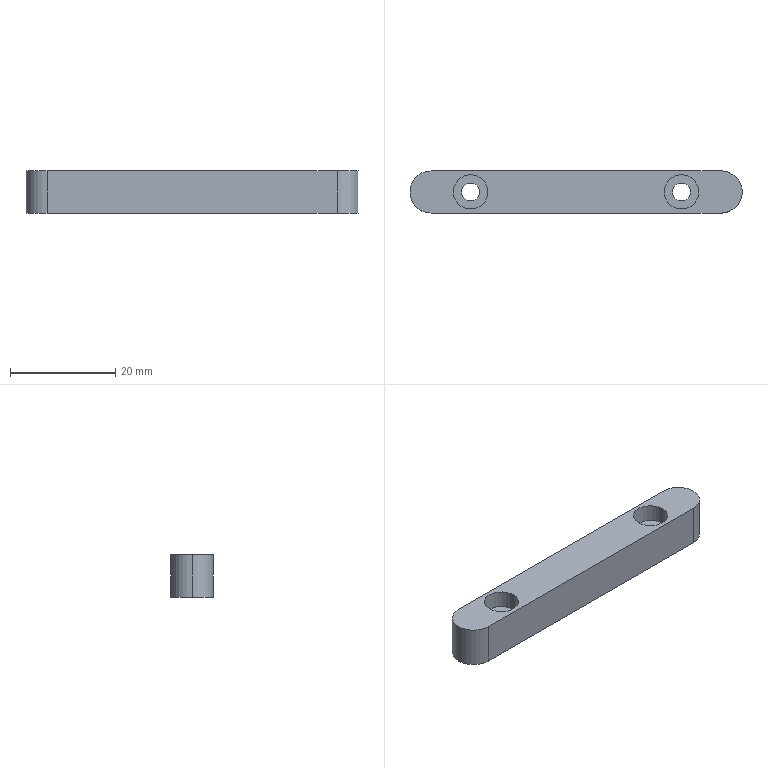Part | SolidWorks | features Extrusion 1, HoleWzd 1 | 1 solid | 17 faces | box 63 x 8 x 8 mm | volume 3613 mm3 | cylinder 11 | plane 6 | commonest cylinder face diameters 3.4 x4 6.5 x4 8 x3
STEP:
#1=CARTESIAN_POINT('',(-23.25,0.,4.6));
#2=VERTEX_POINT('',#1);
#3=CARTESIAN_POINT('',(-16.75,0.,4.6));
#4=VERTEX_POINT('',#3);
#5=CARTESIAN_POINT('',(-20.,0.,4.6));
#6=DIRECTION('',(0.,0.,1.));
#7=DIRECTION('',(1.,0.,0.));
#8=AXIS2_PLACEMENT_3D('',#5,#6,#7);
#9=CIRCLE('',#8,3.25);
#10=EDGE_CURVE('',#2,#4,#9,.T.);
#11=ORIENTED_EDGE('',*,*,#10,.F.);
#12=CARTESIAN_POINT('',(-23.25,0.,8.));
#13=VERTEX_POINT('',#12);
#14=CARTESIAN_POINT('',(-23.25,0.,8.));
#15=DIRECTION('',(0.,0.,1.));
#16=VECTOR('',#15,1000.);
#17=LINE('',#14,#16);
#18=EDGE_CURVE('',#2,#13,#17,.T.);
#19=ORIENTED_EDGE('',*,*,#18,.T.);
#20=CARTESIAN_POINT('',(-16.75,0.,8.));
#21=VERTEX_POINT('',#20);
#22=CARTESIAN_POINT('',(-20.,0.,8.));
#23=DIRECTION('',(0.,0.,1.));
#24=DIRECTION('',(1.,0.,0.));
#25=AXIS2_PLACEMENT_3D('',#22,#23,#24);
#26=CIRCLE('',#25,3.25);
#27=EDGE_CURVE('',#13,#21,#26,.T.);
#28=ORIENTED_EDGE('',*,*,#27,.T.);
#29=CARTESIAN_POINT('',(-16.75,0.,8.));
#30=DIRECTION('',(0.,0.,1.));
#31=VECTOR('',#30,1000.);
#32=LINE('',#29,#31);
#33=EDGE_CURVE('',#4,#21,#32,.T.);
#34=ORIENTED_EDGE('',*,*,#33,.F.);
#35=EDGE_LOOP('',(#11,#19,#28,#34));
#36=FACE_OUTER_BOUND('',#35,.T.);
#37=CARTESIAN_POINT('',(-20.,0.,8.));
#38=DIRECTION('',(0.,0.,1.));
#39=DIRECTION('',(1.,0.,0.));
#40=AXIS2_PLACEMENT_3D('',#37,#38,#39);
#41=CYLINDRICAL_SURFACE('',#40,3.25);
#42=ADVANCED_FACE('',(#36),#41,.F.);
#43=CARTESIAN_POINT('',(-21.7,0.,0.));
#44=VERTEX_POINT('',#43);
#45=CARTESIAN_POINT('',(-18.3,0.,0.));
#46=VERTEX_POINT('',#45);
#47=CARTESIAN_POINT('',(-20.,0.,0.));
#48=DIRECTION('',(0.,0.,1.));
#49=DIRECTION('',(1.,0.,0.));
#50=AXIS2_PLACEMENT_3D('',#47,#48,#49);
#51=CIRCLE('',#50,1.7);
#52=EDGE_CURVE('',#44,#46,#51,.T.);
#53=ORIENTED_EDGE('',*,*,#52,.F.);
#54=CARTESIAN_POINT('',(-21.7,0.,4.6));
#55=VERTEX_POINT('',#54);
#56=CARTESIAN_POINT('',(-21.7,0.,8.));
#57=DIRECTION('',(0.,0.,1.));
#58=VECTOR('',#57,1000.);
#59=LINE('',#56,#58);
#60=EDGE_CURVE('',#44,#55,#59,.T.);
#61=ORIENTED_EDGE('',*,*,#60,.T.);
#62=CARTESIAN_POINT('',(-18.3,0.,4.6));
#63=VERTEX_POINT('',#62);
#64=CARTESIAN_POINT('',(-20.,0.,4.6));
#65=DIRECTION('',(0.,0.,1.));
#66=DIRECTION('',(1.,0.,0.));
#67=AXIS2_PLACEMENT_3D('',#64,#65,#66);
#68=CIRCLE('',#67,1.7);
#69=EDGE_CURVE('',#55,#63,#68,.T.);
#70=ORIENTED_EDGE('',*,*,#69,.T.);
#71=CARTESIAN_POINT('',(-18.3,0.,8.));
#72=DIRECTION('',(0.,0.,1.));
#73=VECTOR('',#72,1000.);
#74=LINE('',#71,#73);
#75=EDGE_CURVE('',#46,#63,#74,.T.);
#76=ORIENTED_EDGE('',*,*,#75,.F.);
#77=EDGE_LOOP('',(#53,#61,#70,#76));
#78=FACE_OUTER_BOUND('',#77,.T.);
#79=CARTESIAN_POINT('',(-20.,0.,8.));
#80=DIRECTION('',(0.,0.,1.));
#81=DIRECTION('',(1.,0.,0.));
#82=AXIS2_PLACEMENT_3D('',#79,#80,#81);
#83=CYLINDRICAL_SURFACE('',#82,1.7);
#84=ADVANCED_FACE('',(#78),#83,.F.);
#85=CARTESIAN_POINT('',(16.75,0.,4.6));
#86=VERTEX_POINT('',#85);
#87=CARTESIAN_POINT('',(23.25,0.,4.6));
#88=VERTEX_POINT('',#87);
#89=CARTESIAN_POINT('',(20.,0.,4.6));
#90=DIRECTION('',(0.,0.,1.));
#91=DIRECTION('',(1.,0.,0.));
#92=AXIS2_PLACEMENT_3D('',#89,#90,#91);
#93=CIRCLE('',#92,3.25);
#94=EDGE_CURVE('',#86,#88,#93,.T.);
#95=ORIENTED_EDGE('',*,*,#94,.F.);
#96=CARTESIAN_POINT('',(16.75,0.,8.));
#97=VERTEX_POINT('',#96);
#98=CARTESIAN_POINT('',(16.75,0.,8.));
#99=DIRECTION('',(0.,0.,1.));
#100=VECTOR('',#99,1000.);
#101=LINE('',#98,#100);
#102=EDGE_CURVE('',#86,#97,#101,.T.);
#103=ORIENTED_EDGE('',*,*,#102,.T.);
#104=CARTESIAN_POINT('',(23.25,0.,8.));
#105=VERTEX_POINT('',#104);
#106=CARTESIAN_POINT('',(20.,0.,8.));
#107=DIRECTION('',(0.,0.,1.));
#108=DIRECTION('',(1.,0.,0.));
#109=AXIS2_PLACEMENT_3D('',#106,#107,#108);
#110=CIRCLE('',#109,3.25);
#111=EDGE_CURVE('',#97,#105,#110,.T.);
#112=ORIENTED_EDGE('',*,*,#111,.T.);
#113=CARTESIAN_POINT('',(23.25,0.,8.));
#114=DIRECTION('',(0.,0.,1.));
#115=VECTOR('',#114,1000.);
#116=LINE('',#113,#115);
#117=EDGE_CURVE('',#88,#105,#116,.T.);
#118=ORIENTED_EDGE('',*,*,#117,.F.);
#119=EDGE_LOOP('',(#95,#103,#112,#118));
#120=FACE_OUTER_BOUND('',#119,.T.);
#121=CARTESIAN_POINT('',(20.,0.,8.));
#122=DIRECTION('',(0.,0.,1.));
#123=DIRECTION('',(1.,0.,0.));
#124=AXIS2_PLACEMENT_3D('',#121,#122,#123);
#125=CYLINDRICAL_SURFACE('',#124,3.25);
#126=ADVANCED_FACE('',(#120),#125,.F.);
#127=CARTESIAN_POINT('',(18.3,0.,0.));
#128=VERTEX_POINT('',#127);
#129=CARTESIAN_POINT('',(21.7,0.,0.));
#130=VERTEX_POINT('',#129);
#131=CARTESIAN_POINT('',(20.,0.,0.));
#132=DIRECTION('',(0.,0.,1.));
#133=DIRECTION('',(1.,0.,0.));
#134=AXIS2_PLACEMENT_3D('',#131,#132,#133);
#135=CIRCLE('',#134,1.7);
#136=EDGE_CURVE('',#128,#130,#135,.T.);
#137=ORIENTED_EDGE('',*,*,#136,.F.);
#138=CARTESIAN_POINT('',(18.3,0.,4.6));
#139=VERTEX_POINT('',#138);
#140=CARTESIAN_POINT('',(18.3,0.,8.));
#141=DIRECTION('',(0.,0.,1.));
#142=VECTOR('',#141,1000.);
#143=LINE('',#140,#142);
#144=EDGE_CURVE('',#128,#139,#143,.T.);
#145=ORIENTED_EDGE('',*,*,#144,.T.);
#146=CARTESIAN_POINT('',(21.7,0.,4.6));
#147=VERTEX_POINT('',#146);
#148=CARTESIAN_POINT('',(20.,0.,4.6));
#149=DIRECTION('',(0.,0.,1.));
#150=DIRECTION('',(1.,0.,0.));
#151=AXIS2_PLACEMENT_3D('',#148,#149,#150);
#152=CIRCLE('',#151,1.7);
#153=EDGE_CURVE('',#139,#147,#152,.T.);
#154=ORIENTED_EDGE('',*,*,#153,.T.);
#155=CARTESIAN_POINT('',(21.7,0.,8.));
#156=DIRECTION('',(0.,0.,1.));
#157=VECTOR('',#156,1000.);
#158=LINE('',#155,#157);
#159=EDGE_CURVE('',#130,#147,#158,.T.);
#160=ORIENTED_EDGE('',*,*,#159,.F.);
#161=EDGE_LOOP('',(#137,#145,#154,#160));
#162=FACE_OUTER_BOUND('',#161,.T.);
#163=CARTESIAN_POINT('',(20.,0.,8.));
#164=DIRECTION('',(0.,0.,1.));
#165=DIRECTION('',(1.,0.,0.));
#166=AXIS2_PLACEMENT_3D('',#163,#164,#165);
#167=CYLINDRICAL_SURFACE('',#166,1.7);
#168=ADVANCED_FACE('',(#162),#167,.F.);
#169=CARTESIAN_POINT('',(-31.5,0.,8.));
#170=VERTEX_POINT('',#169);
#171=CARTESIAN_POINT('',(-27.5,-4.,8.));
#172=VERTEX_POINT('',#171);
#173=CARTESIAN_POINT('',(-27.5,0.,8.));
#174=DIRECTION('',(0.,0.,1.));
#175=DIRECTION('',(1.,0.,0.));
#176=AXIS2_PLACEMENT_3D('',#173,#174,#175);
#177=CIRCLE('',#176,4.);
#178=EDGE_CURVE('',#170,#172,#177,.T.);
#179=ORIENTED_EDGE('',*,*,#178,.F.);
#180=CARTESIAN_POINT('',(-31.5,0.,0.));
#181=VERTEX_POINT('',#180);
#182=CARTESIAN_POINT('',(-31.5,0.,8.));
#183=DIRECTION('',(0.,0.,-1.));
#184=VECTOR('',#183,1000.);
#185=LINE('',#182,#184);
#186=EDGE_CURVE('',#170,#181,#185,.T.);
#187=ORIENTED_EDGE('',*,*,#186,.T.);
#188=CARTESIAN_POINT('',(-27.5,-4.,0.));
#189=VERTEX_POINT('',#188);
#190=CARTESIAN_POINT('',(-27.5,0.,0.));
#191=DIRECTION('',(0.,0.,1.));
#192=DIRECTION('',(1.,0.,0.));
#193=AXIS2_PLACEMENT_3D('',#190,#191,#192);
#194=CIRCLE('',#193,4.);
#195=EDGE_CURVE('',#181,#189,#194,.T.);
#196=ORIENTED_EDGE('',*,*,#195,.T.);
#197=CARTESIAN_POINT('',(-27.5,-4.,8.));
#198=DIRECTION('',(0.,0.,-1.));
#199=VECTOR('',#198,1000.);
#200=LINE('',#197,#199);
#201=EDGE_CURVE('',#172,#189,#200,.T.);
#202=ORIENTED_EDGE('',*,*,#201,.F.);
#203=EDGE_LOOP('',(#179,#187,#196,#202));
#204=FACE_OUTER_BOUND('',#203,.T.);
#205=CARTESIAN_POINT('',(-27.5,0.,8.));
#206=DIRECTION('',(0.,0.,-1.));
#207=DIRECTION('',(-1.,0.,0.));
#208=AXIS2_PLACEMENT_3D('',#205,#206,#207);
#209=CYLINDRICAL_SURFACE('',#208,4.);
#210=ADVANCED_FACE('',(#204),#209,.T.);
#211=ORIENTED_EDGE('',*,*,#186,.F.);
#212=CARTESIAN_POINT('',(-27.5,4.,8.));
#213=VERTEX_POINT('',#212);
#214=CARTESIAN_POINT('',(-27.5,0.,8.));
#215=DIRECTION('',(0.,0.,1.));
#216=DIRECTION('',(1.,0.,0.));
#217=AXIS2_PLACEMENT_3D('',#214,#215,#216);
#218=CIRCLE('',#217,4.);
#219=EDGE_CURVE('',#213,#170,#218,.T.);
#220=ORIENTED_EDGE('',*,*,#219,.F.);
#221=CARTESIAN_POINT('',(-27.5,4.,0.));
#222=VERTEX_POINT('',#221);
#223=CARTESIAN_POINT('',(-27.5,4.,8.));
#224=DIRECTION('',(0.,0.,-1.));
#225=VECTOR('',#224,1000.);
#226=LINE('',#223,#225);
#227=EDGE_CURVE('',#213,#222,#226,.T.);
#228=ORIENTED_EDGE('',*,*,#227,.T.);
#229=CARTESIAN_POINT('',(-27.5,0.,0.));
#230=DIRECTION('',(0.,0.,1.));
#231=DIRECTION('',(1.,0.,0.));
#232=AXIS2_PLACEMENT_3D('',#229,#230,#231);
#233=CIRCLE('',#232,4.);
#234=EDGE_CURVE('',#222,#181,#233,.T.);
#235=ORIENTED_EDGE('',*,*,#234,.T.);
#236=EDGE_LOOP('',(#211,#220,#228,#235));
#237=FACE_OUTER_BOUND('',#236,.T.);
#238=CARTESIAN_POINT('',(-27.5,0.,8.));
#239=DIRECTION('',(0.,0.,-1.));
#240=DIRECTION('',(-1.,0.,0.));
#241=AXIS2_PLACEMENT_3D('',#238,#239,#240);
#242=CYLINDRICAL_SURFACE('',#241,4.);
#243=ADVANCED_FACE('',(#237),#242,.T.);
#244=CARTESIAN_POINT('',(27.5,-4.,0.));
#245=VERTEX_POINT('',#244);
#246=CARTESIAN_POINT('',(-27.5,-4.,0.));
#247=DIRECTION('',(1.,0.,0.));
#248=VECTOR('',#247,1000.);
#249=LINE('',#246,#248);
#250=EDGE_CURVE('',#189,#245,#249,.T.);
#251=ORIENTED_EDGE('',*,*,#250,.T.);
#252=CARTESIAN_POINT('',(27.5,-4.,8.));
#253=VERTEX_POINT('',#252);
#254=CARTESIAN_POINT('',(27.5,-4.,8.));
#255=DIRECTION('',(0.,0.,-1.));
#256=VECTOR('',#255,1000.);
#257=LINE('',#254,#256);
#258=EDGE_CURVE('',#253,#245,#257,.T.);
#259=ORIENTED_EDGE('',*,*,#258,.F.);
#260=CARTESIAN_POINT('',(-27.5,-4.,8.));
#261=DIRECTION('',(1.,0.,0.));
#262=VECTOR('',#261,1000.);
#263=LINE('',#260,#262);
#264=EDGE_CURVE('',#172,#253,#263,.T.);
#265=ORIENTED_EDGE('',*,*,#264,.F.);
#266=ORIENTED_EDGE('',*,*,#201,.T.);
#267=EDGE_LOOP('',(#251,#259,#265,#266));
#268=FACE_OUTER_BOUND('',#267,.T.);
#269=CARTESIAN_POINT('',(-27.5,-4.,8.));
#270=DIRECTION('',(0.,1.,0.));
#271=DIRECTION('',(-1.,0.,0.));
#272=AXIS2_PLACEMENT_3D('',#269,#270,#271);
#273=PLANE('',#272);
#274=ADVANCED_FACE('',(#268),#273,.F.);
#275=CARTESIAN_POINT('',(27.5,4.,0.));
#276=VERTEX_POINT('',#275);
#277=CARTESIAN_POINT('',(27.5,0.,0.));
#278=DIRECTION('',(0.,0.,1.));
#279=DIRECTION('',(1.,0.,0.));
#280=AXIS2_PLACEMENT_3D('',#277,#278,#279);
#281=CIRCLE('',#280,4.);
#282=EDGE_CURVE('',#245,#276,#281,.T.);
#283=ORIENTED_EDGE('',*,*,#282,.T.);
#284=CARTESIAN_POINT('',(27.5,4.,8.));
#285=VERTEX_POINT('',#284);
#286=CARTESIAN_POINT('',(27.5,4.,8.));
#287=DIRECTION('',(0.,0.,-1.));
#288=VECTOR('',#287,1000.);
#289=LINE('',#286,#288);
#290=EDGE_CURVE('',#285,#276,#289,.T.);
#291=ORIENTED_EDGE('',*,*,#290,.F.);
#292=CARTESIAN_POINT('',(27.5,0.,8.));
#293=DIRECTION('',(0.,0.,1.));
#294=DIRECTION('',(1.,0.,0.));
#295=AXIS2_PLACEMENT_3D('',#292,#293,#294);
#296=CIRCLE('',#295,4.);
#297=EDGE_CURVE('',#253,#285,#296,.T.);
#298=ORIENTED_EDGE('',*,*,#297,.F.);
#299=ORIENTED_EDGE('',*,*,#258,.T.);
#300=EDGE_LOOP('',(#283,#291,#298,#299));
#301=FACE_OUTER_BOUND('',#300,.T.);
#302=CARTESIAN_POINT('',(27.5,0.,8.));
#303=DIRECTION('',(0.,0.,-1.));
#304=DIRECTION('',(-1.,0.,0.));
#305=AXIS2_PLACEMENT_3D('',#302,#303,#304);
#306=CYLINDRICAL_SURFACE('',#305,4.);
#307=ADVANCED_FACE('',(#301),#306,.T.);
#308=CARTESIAN_POINT('',(-27.5,4.,0.));
#309=DIRECTION('',(-1.,0.,0.));
#310=VECTOR('',#309,1000.);
#311=LINE('',#308,#310);
#312=EDGE_CURVE('',#276,#222,#311,.T.);
#313=ORIENTED_EDGE('',*,*,#312,.T.);
#314=ORIENTED_EDGE('',*,*,#227,.F.);
#315=CARTESIAN_POINT('',(-27.5,4.,8.));
#316=DIRECTION('',(-1.,0.,0.));
#317=VECTOR('',#316,1000.);
#318=LINE('',#315,#317);
#319=EDGE_CURVE('',#285,#213,#318,.T.);
#320=ORIENTED_EDGE('',*,*,#319,.F.);
#321=ORIENTED_EDGE('',*,*,#290,.T.);
#322=EDGE_LOOP('',(#313,#314,#320,#321));
#323=FACE_OUTER_BOUND('',#322,.T.);
#324=CARTESIAN_POINT('',(-27.5,4.,8.));
#325=DIRECTION('',(0.,-1.,0.));
#326=DIRECTION('',(1.,0.,0.));
#327=AXIS2_PLACEMENT_3D('',#324,#325,#326);
#328=PLANE('',#327);
#329=ADVANCED_FACE('',(#323),#328,.F.);
#330=CARTESIAN_POINT('',(-20.,0.,8.));
#331=DIRECTION('',(0.,0.,1.));
#332=DIRECTION('',(1.,0.,0.));
#333=AXIS2_PLACEMENT_3D('',#330,#331,#332);
#334=CIRCLE('',#333,3.25);
#335=EDGE_CURVE('',#21,#13,#334,.T.);
#336=ORIENTED_EDGE('',*,*,#335,.F.);
#337=ORIENTED_EDGE('',*,*,#27,.F.);
#338=EDGE_LOOP('',(#336,#337));
#339=FACE_BOUND('',#338,.T.);
#340=CARTESIAN_POINT('',(20.,0.,8.));
#341=DIRECTION('',(0.,0.,1.));
#342=DIRECTION('',(1.,0.,0.));
#343=AXIS2_PLACEMENT_3D('',#340,#341,#342);
#344=CIRCLE('',#343,3.25);
#345=EDGE_CURVE('',#105,#97,#344,.T.);
#346=ORIENTED_EDGE('',*,*,#345,.F.);
#347=ORIENTED_EDGE('',*,*,#111,.F.);
#348=EDGE_LOOP('',(#346,#347));
#349=FACE_BOUND('',#348,.T.);
#350=ORIENTED_EDGE('',*,*,#219,.T.);
#351=ORIENTED_EDGE('',*,*,#178,.T.);
#352=ORIENTED_EDGE('',*,*,#264,.T.);
#353=ORIENTED_EDGE('',*,*,#297,.T.);
#354=ORIENTED_EDGE('',*,*,#319,.T.);
#355=EDGE_LOOP('',(#350,#351,#352,#353,#354));
#356=FACE_OUTER_BOUND('',#355,.T.);
#357=CARTESIAN_POINT('',(-27.5,0.,8.));
#358=DIRECTION('',(0.,0.,1.));
#359=DIRECTION('',(1.,0.,0.));
#360=AXIS2_PLACEMENT_3D('',#357,#358,#359);
#361=PLANE('',#360);
#362=ADVANCED_FACE('',(#339,#349,#356),#361,.T.);
#363=CARTESIAN_POINT('',(-20.,0.,0.));
#364=DIRECTION('',(0.,0.,1.));
#365=DIRECTION('',(1.,0.,0.));
#366=AXIS2_PLACEMENT_3D('',#363,#364,#365);
#367=CIRCLE('',#366,1.7);
#368=EDGE_CURVE('',#46,#44,#367,.T.);
#369=ORIENTED_EDGE('',*,*,#368,.T.);
#370=ORIENTED_EDGE('',*,*,#52,.T.);
#371=EDGE_LOOP('',(#369,#370));
#372=FACE_BOUND('',#371,.T.);
#373=CARTESIAN_POINT('',(20.,0.,0.));
#374=DIRECTION('',(0.,0.,1.));
#375=DIRECTION('',(1.,0.,0.));
#376=AXIS2_PLACEMENT_3D('',#373,#374,#375);
#377=CIRCLE('',#376,1.7);
#378=EDGE_CURVE('',#130,#128,#377,.T.);
#379=ORIENTED_EDGE('',*,*,#378,.T.);
#380=ORIENTED_EDGE('',*,*,#136,.T.);
#381=EDGE_LOOP('',(#379,#380));
#382=FACE_BOUND('',#381,.T.);
#383=ORIENTED_EDGE('',*,*,#234,.F.);
#384=ORIENTED_EDGE('',*,*,#312,.F.);
#385=ORIENTED_EDGE('',*,*,#282,.F.);
#386=ORIENTED_EDGE('',*,*,#250,.F.);
#387=ORIENTED_EDGE('',*,*,#195,.F.);
#388=EDGE_LOOP('',(#383,#384,#385,#386,#387));
#389=FACE_OUTER_BOUND('',#388,.T.);
#390=CARTESIAN_POINT('',(-27.5,0.,0.));
#391=DIRECTION('',(0.,0.,1.));
#392=DIRECTION('',(1.,0.,0.));
#393=AXIS2_PLACEMENT_3D('',#390,#391,#392);
#394=PLANE('',#393);
#395=ADVANCED_FACE('',(#372,#382,#389),#394,.F.);
#396=ORIENTED_EDGE('',*,*,#144,.F.);
#397=ORIENTED_EDGE('',*,*,#378,.F.);
#398=ORIENTED_EDGE('',*,*,#159,.T.);
#399=CARTESIAN_POINT('',(20.,0.,4.6));
#400=DIRECTION('',(0.,0.,1.));
#401=DIRECTION('',(1.,0.,0.));
#402=AXIS2_PLACEMENT_3D('',#399,#400,#401);
#403=CIRCLE('',#402,1.7);
#404=EDGE_CURVE('',#147,#139,#403,.T.);
#405=ORIENTED_EDGE('',*,*,#404,.T.);
#406=EDGE_LOOP('',(#396,#397,#398,#405));
#407=FACE_OUTER_BOUND('',#406,.T.);
#408=CARTESIAN_POINT('',(20.,0.,8.));
#409=DIRECTION('',(0.,0.,1.));
#410=DIRECTION('',(1.,0.,0.));
#411=AXIS2_PLACEMENT_3D('',#408,#409,#410);
#412=CYLINDRICAL_SURFACE('',#411,1.7);
#413=ADVANCED_FACE('',(#407),#412,.F.);
#414=ORIENTED_EDGE('',*,*,#404,.F.);
#415=ORIENTED_EDGE('',*,*,#153,.F.);
#416=EDGE_LOOP('',(#414,#415));
#417=FACE_BOUND('',#416,.T.);
#418=CARTESIAN_POINT('',(20.,0.,4.6));
#419=DIRECTION('',(0.,0.,1.));
#420=DIRECTION('',(1.,0.,0.));
#421=AXIS2_PLACEMENT_3D('',#418,#419,#420);
#422=CIRCLE('',#421,3.25);
#423=EDGE_CURVE('',#88,#86,#422,.T.);
#424=ORIENTED_EDGE('',*,*,#423,.T.);
#425=ORIENTED_EDGE('',*,*,#94,.T.);
#426=EDGE_LOOP('',(#424,#425));
#427=FACE_OUTER_BOUND('',#426,.T.);
#428=CARTESIAN_POINT('',(21.7,0.,4.6));
#429=DIRECTION('',(0.,0.,-1.));
#430=DIRECTION('',(-1.,0.,0.));
#431=AXIS2_PLACEMENT_3D('',#428,#429,#430);
#432=PLANE('',#431);
#433=ADVANCED_FACE('',(#417,#427),#432,.F.);
#434=ORIENTED_EDGE('',*,*,#102,.F.);
#435=ORIENTED_EDGE('',*,*,#423,.F.);
#436=ORIENTED_EDGE('',*,*,#117,.T.);
#437=ORIENTED_EDGE('',*,*,#345,.T.);
#438=EDGE_LOOP('',(#434,#435,#436,#437));
#439=FACE_OUTER_BOUND('',#438,.T.);
#440=CARTESIAN_POINT('',(20.,0.,8.));
#441=DIRECTION('',(0.,0.,1.));
#442=DIRECTION('',(1.,0.,0.));
#443=AXIS2_PLACEMENT_3D('',#440,#441,#442);
#444=CYLINDRICAL_SURFACE('',#443,3.25);
#445=ADVANCED_FACE('',(#439),#444,.F.);
#446=ORIENTED_EDGE('',*,*,#60,.F.);
#447=ORIENTED_EDGE('',*,*,#368,.F.);
#448=ORIENTED_EDGE('',*,*,#75,.T.);
#449=CARTESIAN_POINT('',(-20.,0.,4.6));
#450=DIRECTION('',(0.,0.,1.));
#451=DIRECTION('',(1.,0.,0.));
#452=AXIS2_PLACEMENT_3D('',#449,#450,#451);
#453=CIRCLE('',#452,1.7);
#454=EDGE_CURVE('',#63,#55,#453,.T.);
#455=ORIENTED_EDGE('',*,*,#454,.T.);
#456=EDGE_LOOP('',(#446,#447,#448,#455));
#457=FACE_OUTER_BOUND('',#456,.T.);
#458=CARTESIAN_POINT('',(-20.,0.,8.));
#459=DIRECTION('',(0.,0.,1.));
#460=DIRECTION('',(1.,0.,0.));
#461=AXIS2_PLACEMENT_3D('',#458,#459,#460);
#462=CYLINDRICAL_SURFACE('',#461,1.7);
#463=ADVANCED_FACE('',(#457),#462,.F.);
#464=ORIENTED_EDGE('',*,*,#454,.F.);
#465=ORIENTED_EDGE('',*,*,#69,.F.);
#466=EDGE_LOOP('',(#464,#465));
#467=FACE_BOUND('',#466,.T.);
#468=CARTESIAN_POINT('',(-20.,0.,4.6));
#469=DIRECTION('',(0.,0.,1.));
#470=DIRECTION('',(1.,0.,0.));
#471=AXIS2_PLACEMENT_3D('',#468,#469,#470);
#472=CIRCLE('',#471,3.25);
#473=EDGE_CURVE('',#4,#2,#472,.T.);
#474=ORIENTED_EDGE('',*,*,#473,.T.);
#475=ORIENTED_EDGE('',*,*,#10,.T.);
#476=EDGE_LOOP('',(#474,#475));
#477=FACE_OUTER_BOUND('',#476,.T.);
#478=CARTESIAN_POINT('',(-18.3,0.,4.6));
#479=DIRECTION('',(0.,0.,-1.));
#480=DIRECTION('',(-1.,0.,0.));
#481=AXIS2_PLACEMENT_3D('',#478,#479,#480);
#482=PLANE('',#481);
#483=ADVANCED_FACE('',(#467,#477),#482,.F.);
#484=ORIENTED_EDGE('',*,*,#18,.F.);
#485=ORIENTED_EDGE('',*,*,#473,.F.);
#486=ORIENTED_EDGE('',*,*,#33,.T.);
#487=ORIENTED_EDGE('',*,*,#335,.T.);
#488=EDGE_LOOP('',(#484,#485,#486,#487));
#489=FACE_OUTER_BOUND('',#488,.T.);
#490=CARTESIAN_POINT('',(-20.,0.,8.));
#491=DIRECTION('',(0.,0.,1.));
#492=DIRECTION('',(1.,0.,0.));
#493=AXIS2_PLACEMENT_3D('',#490,#491,#492);
#494=CYLINDRICAL_SURFACE('',#493,3.25);
#495=ADVANCED_FACE('',(#489),#494,.F.);
#496=CLOSED_SHELL('',(#42,#84,#126,#168,#210,#243,#274,#307,#329,#362,#395,#413,#433,#445,#463,#483,#495));
#497=MANIFOLD_SOLID_BREP('',#496);
#498=CARTESIAN_POINT('',(0.,0.,0.));
#499=DIRECTION('',(0.,0.,1.));
#500=DIRECTION('',(1.,0.,0.));
#501=AXIS2_PLACEMENT_3D('',#498,#499,#500);
#502=(LENGTH_UNIT()NAMED_UNIT(*)SI_UNIT(.MILLI.,.METRE.));
#503=UNCERTAINTY_MEASURE_WITH_UNIT(LENGTH_MEASURE(0.00001),#502,'','');
#504=(NAMED_UNIT(*)PLANE_ANGLE_UNIT()SI_UNIT($,.RADIAN.));
#505=(NAMED_UNIT(*)SI_UNIT($,.STERADIAN.)SOLID_ANGLE_UNIT());
#506=(GEOMETRIC_REPRESENTATION_CONTEXT(3)GLOBAL_UNCERTAINTY_ASSIGNED_CONTEXT((#503))GLOBAL_UNIT_ASSIGNED_CONTEXT((#502,#504,#505))REPRESENTATION_CONTEXT('',''));
#507=ADVANCED_BREP_SHAPE_REPRESENTATION('',(#497,#501),#506);